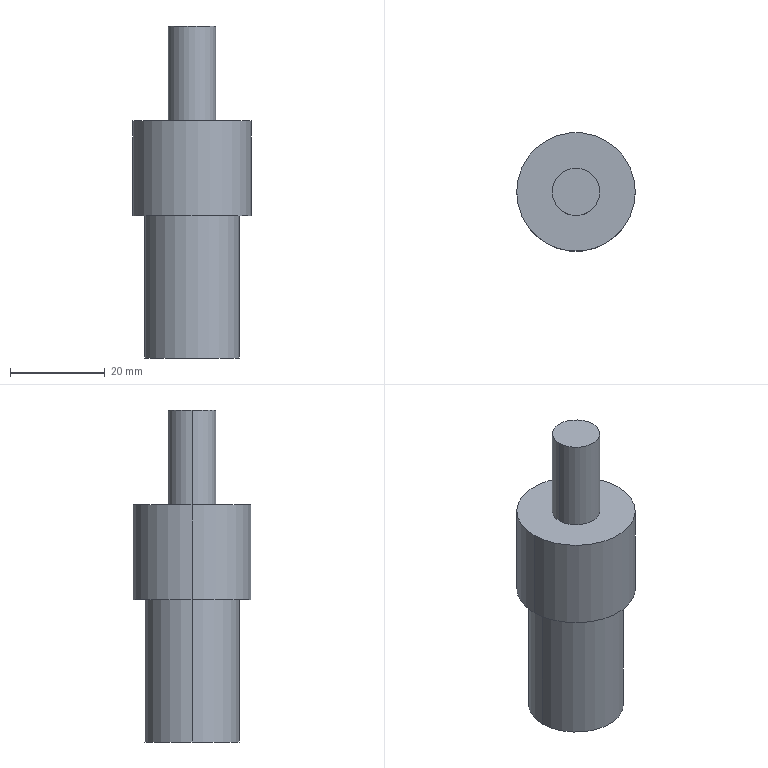Part | SolidWorks | features ICE 2, Extrusion 1 | 1 solid | 10 faces | box 25 x 25 x 70 mm | volume 20813 mm3 | cylinder 6 | plane 4 | commonest cylinder face diameters 10 x2 20 x2 25 x2
STEP:
#1=CARTESIAN_POINT('',(5.,0.,70.));
#2=VERTEX_POINT('',#1);
#3=CARTESIAN_POINT('',(-5.,0.,70.));
#4=VERTEX_POINT('',#3);
#5=CARTESIAN_POINT('',(0.,0.,70.));
#6=DIRECTION('',(0.,0.,1.));
#7=DIRECTION('',(1.,0.,0.));
#8=AXIS2_PLACEMENT_3D('',#5,#6,#7);
#9=CIRCLE('',#8,5.);
#10=EDGE_CURVE('',#2,#4,#9,.T.);
#11=ORIENTED_EDGE('',*,*,#10,.F.);
#12=CARTESIAN_POINT('',(5.,0.,50.));
#13=VERTEX_POINT('',#12);
#14=CARTESIAN_POINT('',(5.,0.,70.));
#15=DIRECTION('',(0.,0.,-1.));
#16=VECTOR('',#15,1000.);
#17=LINE('',#14,#16);
#18=EDGE_CURVE('',#2,#13,#17,.T.);
#19=ORIENTED_EDGE('',*,*,#18,.T.);
#20=CARTESIAN_POINT('',(-5.,0.,50.));
#21=VERTEX_POINT('',#20);
#22=CARTESIAN_POINT('',(0.,0.,50.));
#23=DIRECTION('',(0.,0.,1.));
#24=DIRECTION('',(1.,0.,0.));
#25=AXIS2_PLACEMENT_3D('',#22,#23,#24);
#26=CIRCLE('',#25,5.);
#27=EDGE_CURVE('',#13,#21,#26,.T.);
#28=ORIENTED_EDGE('',*,*,#27,.T.);
#29=CARTESIAN_POINT('',(-5.,0.,70.));
#30=DIRECTION('',(0.,0.,-1.));
#31=VECTOR('',#30,1000.);
#32=LINE('',#29,#31);
#33=EDGE_CURVE('',#4,#21,#32,.T.);
#34=ORIENTED_EDGE('',*,*,#33,.F.);
#35=EDGE_LOOP('',(#11,#19,#28,#34));
#36=FACE_OUTER_BOUND('',#35,.T.);
#37=CARTESIAN_POINT('',(0.,0.,70.));
#38=DIRECTION('',(0.,0.,-1.));
#39=DIRECTION('',(-1.,0.,0.));
#40=AXIS2_PLACEMENT_3D('',#37,#38,#39);
#41=CYLINDRICAL_SURFACE('',#40,5.);
#42=ADVANCED_FACE('',(#36),#41,.T.);
#43=CARTESIAN_POINT('',(12.5,0.,50.));
#44=VERTEX_POINT('',#43);
#45=CARTESIAN_POINT('',(-12.5,0.,50.));
#46=VERTEX_POINT('',#45);
#47=CARTESIAN_POINT('',(0.,0.,50.));
#48=DIRECTION('',(0.,0.,1.));
#49=DIRECTION('',(1.,0.,0.));
#50=AXIS2_PLACEMENT_3D('',#47,#48,#49);
#51=CIRCLE('',#50,12.5);
#52=EDGE_CURVE('',#44,#46,#51,.T.);
#53=ORIENTED_EDGE('',*,*,#52,.F.);
#54=CARTESIAN_POINT('',(12.5,0.,30.));
#55=VERTEX_POINT('',#54);
#56=CARTESIAN_POINT('',(12.5,0.,50.));
#57=DIRECTION('',(0.,0.,-1.));
#58=VECTOR('',#57,1000.);
#59=LINE('',#56,#58);
#60=EDGE_CURVE('',#44,#55,#59,.T.);
#61=ORIENTED_EDGE('',*,*,#60,.T.);
#62=CARTESIAN_POINT('',(-12.5,0.,30.));
#63=VERTEX_POINT('',#62);
#64=CARTESIAN_POINT('',(0.,0.,30.));
#65=DIRECTION('',(0.,0.,1.));
#66=DIRECTION('',(1.,0.,0.));
#67=AXIS2_PLACEMENT_3D('',#64,#65,#66);
#68=CIRCLE('',#67,12.5);
#69=EDGE_CURVE('',#55,#63,#68,.T.);
#70=ORIENTED_EDGE('',*,*,#69,.T.);
#71=CARTESIAN_POINT('',(-12.5,0.,50.));
#72=DIRECTION('',(0.,0.,-1.));
#73=VECTOR('',#72,1000.);
#74=LINE('',#71,#73);
#75=EDGE_CURVE('',#46,#63,#74,.T.);
#76=ORIENTED_EDGE('',*,*,#75,.F.);
#77=EDGE_LOOP('',(#53,#61,#70,#76));
#78=FACE_OUTER_BOUND('',#77,.T.);
#79=CARTESIAN_POINT('',(0.,0.,50.));
#80=DIRECTION('',(0.,0.,-1.));
#81=DIRECTION('',(-1.,0.,0.));
#82=AXIS2_PLACEMENT_3D('',#79,#80,#81);
#83=CYLINDRICAL_SURFACE('',#82,12.5);
#84=ADVANCED_FACE('',(#78),#83,.T.);
#85=CARTESIAN_POINT('',(10.,0.,30.));
#86=VERTEX_POINT('',#85);
#87=CARTESIAN_POINT('',(-10.,0.,30.));
#88=VERTEX_POINT('',#87);
#89=CARTESIAN_POINT('',(0.,0.,30.));
#90=DIRECTION('',(0.,0.,1.));
#91=DIRECTION('',(1.,0.,0.));
#92=AXIS2_PLACEMENT_3D('',#89,#90,#91);
#93=CIRCLE('',#92,10.);
#94=EDGE_CURVE('',#86,#88,#93,.T.);
#95=ORIENTED_EDGE('',*,*,#94,.F.);
#96=CARTESIAN_POINT('',(10.,0.,0.));
#97=VERTEX_POINT('',#96);
#98=CARTESIAN_POINT('',(10.,0.,30.));
#99=DIRECTION('',(0.,0.,-1.));
#100=VECTOR('',#99,1000.);
#101=LINE('',#98,#100);
#102=EDGE_CURVE('',#86,#97,#101,.T.);
#103=ORIENTED_EDGE('',*,*,#102,.T.);
#104=CARTESIAN_POINT('',(-10.,0.,0.));
#105=VERTEX_POINT('',#104);
#106=CARTESIAN_POINT('',(0.,0.,0.));
#107=DIRECTION('',(0.,0.,1.));
#108=DIRECTION('',(1.,0.,0.));
#109=AXIS2_PLACEMENT_3D('',#106,#107,#108);
#110=CIRCLE('',#109,10.);
#111=EDGE_CURVE('',#97,#105,#110,.T.);
#112=ORIENTED_EDGE('',*,*,#111,.T.);
#113=CARTESIAN_POINT('',(-10.,0.,30.));
#114=DIRECTION('',(0.,0.,-1.));
#115=VECTOR('',#114,1000.);
#116=LINE('',#113,#115);
#117=EDGE_CURVE('',#88,#105,#116,.T.);
#118=ORIENTED_EDGE('',*,*,#117,.F.);
#119=EDGE_LOOP('',(#95,#103,#112,#118));
#120=FACE_OUTER_BOUND('',#119,.T.);
#121=CARTESIAN_POINT('',(0.,0.,30.));
#122=DIRECTION('',(0.,0.,-1.));
#123=DIRECTION('',(-1.,0.,0.));
#124=AXIS2_PLACEMENT_3D('',#121,#122,#123);
#125=CYLINDRICAL_SURFACE('',#124,10.);
#126=ADVANCED_FACE('',(#120),#125,.T.);
#127=ORIENTED_EDGE('',*,*,#102,.F.);
#128=CARTESIAN_POINT('',(0.,0.,30.));
#129=DIRECTION('',(0.,0.,1.));
#130=DIRECTION('',(1.,0.,0.));
#131=AXIS2_PLACEMENT_3D('',#128,#129,#130);
#132=CIRCLE('',#131,10.);
#133=EDGE_CURVE('',#88,#86,#132,.T.);
#134=ORIENTED_EDGE('',*,*,#133,.F.);
#135=ORIENTED_EDGE('',*,*,#117,.T.);
#136=CARTESIAN_POINT('',(0.,0.,0.));
#137=DIRECTION('',(0.,0.,1.));
#138=DIRECTION('',(1.,0.,0.));
#139=AXIS2_PLACEMENT_3D('',#136,#137,#138);
#140=CIRCLE('',#139,10.);
#141=EDGE_CURVE('',#105,#97,#140,.T.);
#142=ORIENTED_EDGE('',*,*,#141,.T.);
#143=EDGE_LOOP('',(#127,#134,#135,#142));
#144=FACE_OUTER_BOUND('',#143,.T.);
#145=CARTESIAN_POINT('',(0.,0.,30.));
#146=DIRECTION('',(0.,0.,-1.));
#147=DIRECTION('',(-1.,0.,0.));
#148=AXIS2_PLACEMENT_3D('',#145,#146,#147);
#149=CYLINDRICAL_SURFACE('',#148,10.);
#150=ADVANCED_FACE('',(#144),#149,.T.);
#151=ORIENTED_EDGE('',*,*,#141,.F.);
#152=ORIENTED_EDGE('',*,*,#111,.F.);
#153=EDGE_LOOP('',(#151,#152));
#154=FACE_OUTER_BOUND('',#153,.T.);
#155=CARTESIAN_POINT('',(0.,0.,0.));
#156=DIRECTION('',(0.,0.,1.));
#157=DIRECTION('',(1.,0.,0.));
#158=AXIS2_PLACEMENT_3D('',#155,#156,#157);
#159=PLANE('',#158);
#160=ADVANCED_FACE('',(#154),#159,.F.);
#161=ORIENTED_EDGE('',*,*,#60,.F.);
#162=CARTESIAN_POINT('',(0.,0.,50.));
#163=DIRECTION('',(0.,0.,1.));
#164=DIRECTION('',(1.,0.,0.));
#165=AXIS2_PLACEMENT_3D('',#162,#163,#164);
#166=CIRCLE('',#165,12.5);
#167=EDGE_CURVE('',#46,#44,#166,.T.);
#168=ORIENTED_EDGE('',*,*,#167,.F.);
#169=ORIENTED_EDGE('',*,*,#75,.T.);
#170=CARTESIAN_POINT('',(0.,0.,30.));
#171=DIRECTION('',(0.,0.,1.));
#172=DIRECTION('',(1.,0.,0.));
#173=AXIS2_PLACEMENT_3D('',#170,#171,#172);
#174=CIRCLE('',#173,12.5);
#175=EDGE_CURVE('',#63,#55,#174,.T.);
#176=ORIENTED_EDGE('',*,*,#175,.T.);
#177=EDGE_LOOP('',(#161,#168,#169,#176));
#178=FACE_OUTER_BOUND('',#177,.T.);
#179=CARTESIAN_POINT('',(0.,0.,50.));
#180=DIRECTION('',(0.,0.,-1.));
#181=DIRECTION('',(-1.,0.,0.));
#182=AXIS2_PLACEMENT_3D('',#179,#180,#181);
#183=CYLINDRICAL_SURFACE('',#182,12.5);
#184=ADVANCED_FACE('',(#178),#183,.T.);
#185=CARTESIAN_POINT('',(0.,0.,50.));
#186=DIRECTION('',(0.,0.,1.));
#187=DIRECTION('',(1.,0.,0.));
#188=AXIS2_PLACEMENT_3D('',#185,#186,#187);
#189=CIRCLE('',#188,5.);
#190=EDGE_CURVE('',#21,#13,#189,.T.);
#191=ORIENTED_EDGE('',*,*,#190,.F.);
#192=ORIENTED_EDGE('',*,*,#27,.F.);
#193=EDGE_LOOP('',(#191,#192));
#194=FACE_BOUND('',#193,.T.);
#195=ORIENTED_EDGE('',*,*,#167,.T.);
#196=ORIENTED_EDGE('',*,*,#52,.T.);
#197=EDGE_LOOP('',(#195,#196));
#198=FACE_OUTER_BOUND('',#197,.T.);
#199=CARTESIAN_POINT('',(0.,0.,50.));
#200=DIRECTION('',(0.,0.,1.));
#201=DIRECTION('',(1.,0.,0.));
#202=AXIS2_PLACEMENT_3D('',#199,#200,#201);
#203=PLANE('',#202);
#204=ADVANCED_FACE('',(#194,#198),#203,.T.);
#205=ORIENTED_EDGE('',*,*,#133,.T.);
#206=ORIENTED_EDGE('',*,*,#94,.T.);
#207=EDGE_LOOP('',(#205,#206));
#208=FACE_BOUND('',#207,.T.);
#209=ORIENTED_EDGE('',*,*,#175,.F.);
#210=ORIENTED_EDGE('',*,*,#69,.F.);
#211=EDGE_LOOP('',(#209,#210));
#212=FACE_OUTER_BOUND('',#211,.T.);
#213=CARTESIAN_POINT('',(0.,0.,30.));
#214=DIRECTION('',(0.,0.,1.));
#215=DIRECTION('',(1.,0.,0.));
#216=AXIS2_PLACEMENT_3D('',#213,#214,#215);
#217=PLANE('',#216);
#218=ADVANCED_FACE('',(#208,#212),#217,.F.);
#219=ORIENTED_EDGE('',*,*,#18,.F.);
#220=CARTESIAN_POINT('',(0.,0.,70.));
#221=DIRECTION('',(0.,0.,1.));
#222=DIRECTION('',(1.,0.,0.));
#223=AXIS2_PLACEMENT_3D('',#220,#221,#222);
#224=CIRCLE('',#223,5.);
#225=EDGE_CURVE('',#4,#2,#224,.T.);
#226=ORIENTED_EDGE('',*,*,#225,.F.);
#227=ORIENTED_EDGE('',*,*,#33,.T.);
#228=ORIENTED_EDGE('',*,*,#190,.T.);
#229=EDGE_LOOP('',(#219,#226,#227,#228));
#230=FACE_OUTER_BOUND('',#229,.T.);
#231=CARTESIAN_POINT('',(0.,0.,70.));
#232=DIRECTION('',(0.,0.,-1.));
#233=DIRECTION('',(-1.,0.,0.));
#234=AXIS2_PLACEMENT_3D('',#231,#232,#233);
#235=CYLINDRICAL_SURFACE('',#234,5.);
#236=ADVANCED_FACE('',(#230),#235,.T.);
#237=ORIENTED_EDGE('',*,*,#225,.T.);
#238=ORIENTED_EDGE('',*,*,#10,.T.);
#239=EDGE_LOOP('',(#237,#238));
#240=FACE_OUTER_BOUND('',#239,.T.);
#241=CARTESIAN_POINT('',(0.,0.,70.));
#242=DIRECTION('',(0.,0.,1.));
#243=DIRECTION('',(1.,0.,0.));
#244=AXIS2_PLACEMENT_3D('',#241,#242,#243);
#245=PLANE('',#244);
#246=ADVANCED_FACE('',(#240),#245,.T.);
#247=CLOSED_SHELL('',(#42,#84,#126,#150,#160,#184,#204,#218,#236,#246));
#248=MANIFOLD_SOLID_BREP('',#247);
#249=CARTESIAN_POINT('',(0.,0.,0.));
#250=DIRECTION('',(0.,0.,1.));
#251=DIRECTION('',(1.,0.,0.));
#252=AXIS2_PLACEMENT_3D('',#249,#250,#251);
#253=(LENGTH_UNIT()NAMED_UNIT(*)SI_UNIT(.MILLI.,.METRE.));
#254=UNCERTAINTY_MEASURE_WITH_UNIT(LENGTH_MEASURE(0.00001),#253,'','');
#255=(NAMED_UNIT(*)PLANE_ANGLE_UNIT()SI_UNIT($,.RADIAN.));
#256=(NAMED_UNIT(*)SI_UNIT($,.STERADIAN.)SOLID_ANGLE_UNIT());
#257=(GEOMETRIC_REPRESENTATION_CONTEXT(3)GLOBAL_UNCERTAINTY_ASSIGNED_CONTEXT((#254))GLOBAL_UNIT_ASSIGNED_CONTEXT((#253,#255,#256))REPRESENTATION_CONTEXT('',''));
#258=ADVANCED_BREP_SHAPE_REPRESENTATION('',(#248,#252),#257);